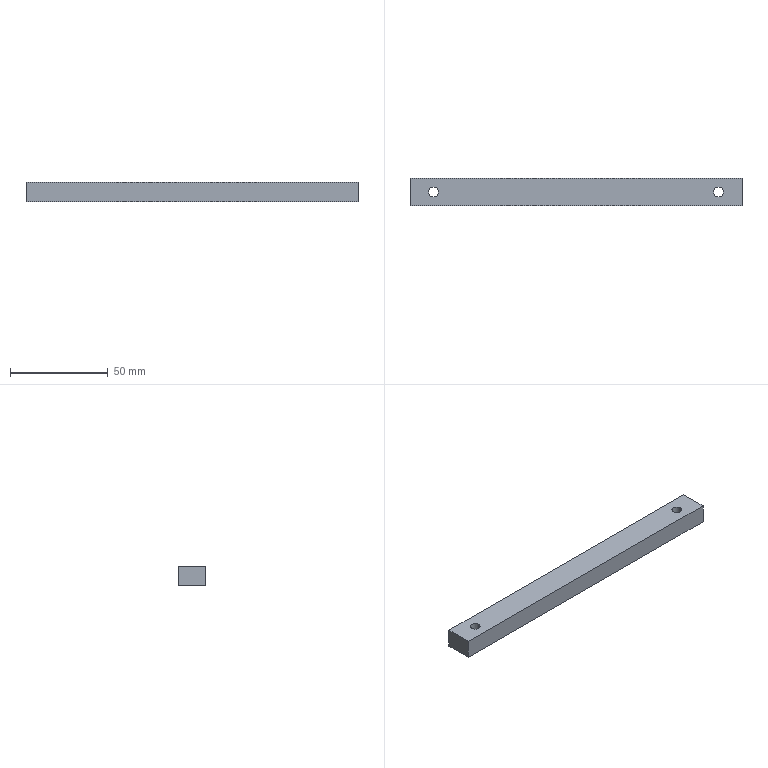Part | SolidWorks | features 3DProfileFeature 1, Extrusion 1, HoleWzd 1, MirrorPattern 1 | 1 solid | 14 faces | box 170 x 14 x 10 mm | volume 23403 mm3 | plane 6 | cone 4 | cylinder 4 | commonest cylinder face diameters 5 x4
STEP:
#1=CARTESIAN_POINT('',(75.5,0.,-4.475));
#2=VERTEX_POINT('',#1);
#3=CARTESIAN_POINT('',(70.5,0.,-4.475));
#4=VERTEX_POINT('',#3);
#5=CARTESIAN_POINT('',(73.,0.,-4.475));
#6=DIRECTION('',(0.,0.,-1.));
#7=DIRECTION('',(-1.,0.,0.));
#8=AXIS2_PLACEMENT_3D('',#5,#6,#7);
#9=CIRCLE('',#8,2.5);
#10=EDGE_CURVE('',#2,#4,#9,.T.);
#11=ORIENTED_EDGE('',*,*,#10,.F.);
#12=CARTESIAN_POINT('',(76.025,0.,-5.));
#13=VERTEX_POINT('',#12);
#14=CARTESIAN_POINT('',(76.025,0.,-5.));
#15=DIRECTION('',(0.7071,0.,-0.7071));
#16=VECTOR('',#15,1000.);
#17=LINE('',#14,#16);
#18=EDGE_CURVE('',#2,#13,#17,.T.);
#19=ORIENTED_EDGE('',*,*,#18,.T.);
#20=CARTESIAN_POINT('',(69.975,0.,-5.));
#21=VERTEX_POINT('',#20);
#22=CARTESIAN_POINT('',(73.,0.,-5.));
#23=DIRECTION('',(0.,0.,-1.));
#24=DIRECTION('',(-1.,0.,0.));
#25=AXIS2_PLACEMENT_3D('',#22,#23,#24);
#26=CIRCLE('',#25,3.025);
#27=EDGE_CURVE('',#13,#21,#26,.T.);
#28=ORIENTED_EDGE('',*,*,#27,.T.);
#29=CARTESIAN_POINT('',(69.975,0.,-5.));
#30=DIRECTION('',(-0.7071,0.,-0.7071));
#31=VECTOR('',#30,1000.);
#32=LINE('',#29,#31);
#33=EDGE_CURVE('',#4,#21,#32,.T.);
#34=ORIENTED_EDGE('',*,*,#33,.F.);
#35=EDGE_LOOP('',(#11,#19,#28,#34));
#36=FACE_OUTER_BOUND('',#35,.T.);
#37=CARTESIAN_POINT('',(73.,0.,-5.));
#38=DIRECTION('',(0.,0.,-1.));
#39=DIRECTION('',(-1.,0.,0.));
#40=AXIS2_PLACEMENT_3D('',#37,#38,#39);
#41=CONICAL_SURFACE('',#40,3.025,0.7854);
#42=ADVANCED_FACE('',(#36),#41,.F.);
#43=CARTESIAN_POINT('',(75.5,0.,5.));
#44=VERTEX_POINT('',#43);
#45=CARTESIAN_POINT('',(70.5,0.,5.));
#46=VERTEX_POINT('',#45);
#47=CARTESIAN_POINT('',(73.,0.,5.));
#48=DIRECTION('',(0.,0.,-1.));
#49=DIRECTION('',(-1.,0.,0.));
#50=AXIS2_PLACEMENT_3D('',#47,#48,#49);
#51=CIRCLE('',#50,2.5);
#52=EDGE_CURVE('',#44,#46,#51,.T.);
#53=ORIENTED_EDGE('',*,*,#52,.F.);
#54=CARTESIAN_POINT('',(75.5,0.,-5.));
#55=DIRECTION('',(0.,0.,-1.));
#56=VECTOR('',#55,1000.);
#57=LINE('',#54,#56);
#58=EDGE_CURVE('',#44,#2,#57,.T.);
#59=ORIENTED_EDGE('',*,*,#58,.T.);
#60=ORIENTED_EDGE('',*,*,#10,.T.);
#61=CARTESIAN_POINT('',(70.5,0.,-5.));
#62=DIRECTION('',(0.,0.,-1.));
#63=VECTOR('',#62,1000.);
#64=LINE('',#61,#63);
#65=EDGE_CURVE('',#46,#4,#64,.T.);
#66=ORIENTED_EDGE('',*,*,#65,.F.);
#67=EDGE_LOOP('',(#53,#59,#60,#66));
#68=FACE_OUTER_BOUND('',#67,.T.);
#69=CARTESIAN_POINT('',(73.,0.,-5.));
#70=DIRECTION('',(0.,0.,-1.));
#71=DIRECTION('',(-1.,0.,0.));
#72=AXIS2_PLACEMENT_3D('',#69,#70,#71);
#73=CYLINDRICAL_SURFACE('',#72,2.5);
#74=ADVANCED_FACE('',(#68),#73,.F.);
#75=CARTESIAN_POINT('',(-70.5,0.,-4.475));
#76=VERTEX_POINT('',#75);
#77=CARTESIAN_POINT('',(-75.5,0.,-4.475));
#78=VERTEX_POINT('',#77);
#79=CARTESIAN_POINT('',(-73.,0.,-4.475));
#80=DIRECTION('',(0.,0.,-1.));
#81=DIRECTION('',(-1.,0.,0.));
#82=AXIS2_PLACEMENT_3D('',#79,#80,#81);
#83=CIRCLE('',#82,2.5);
#84=EDGE_CURVE('',#76,#78,#83,.T.);
#85=ORIENTED_EDGE('',*,*,#84,.F.);
#86=CARTESIAN_POINT('',(-69.975,0.,-5.));
#87=VERTEX_POINT('',#86);
#88=CARTESIAN_POINT('',(-69.975,0.,-5.));
#89=DIRECTION('',(0.7071,0.,-0.7071));
#90=VECTOR('',#89,1000.);
#91=LINE('',#88,#90);
#92=EDGE_CURVE('',#76,#87,#91,.T.);
#93=ORIENTED_EDGE('',*,*,#92,.T.);
#94=CARTESIAN_POINT('',(-76.025,0.,-5.));
#95=VERTEX_POINT('',#94);
#96=CARTESIAN_POINT('',(-73.,0.,-5.));
#97=DIRECTION('',(0.,0.,-1.));
#98=DIRECTION('',(-1.,0.,0.));
#99=AXIS2_PLACEMENT_3D('',#96,#97,#98);
#100=CIRCLE('',#99,3.025);
#101=EDGE_CURVE('',#87,#95,#100,.T.);
#102=ORIENTED_EDGE('',*,*,#101,.T.);
#103=CARTESIAN_POINT('',(-76.025,0.,-5.));
#104=DIRECTION('',(-0.7071,0.,-0.7071));
#105=VECTOR('',#104,1000.);
#106=LINE('',#103,#105);
#107=EDGE_CURVE('',#78,#95,#106,.T.);
#108=ORIENTED_EDGE('',*,*,#107,.F.);
#109=EDGE_LOOP('',(#85,#93,#102,#108));
#110=FACE_OUTER_BOUND('',#109,.T.);
#111=CARTESIAN_POINT('',(-73.,0.,-5.));
#112=DIRECTION('',(0.,0.,-1.));
#113=DIRECTION('',(-1.,0.,0.));
#114=AXIS2_PLACEMENT_3D('',#111,#112,#113);
#115=CONICAL_SURFACE('',#114,3.025,0.7854);
#116=ADVANCED_FACE('',(#110),#115,.F.);
#117=CARTESIAN_POINT('',(-70.5,0.,5.));
#118=VERTEX_POINT('',#117);
#119=CARTESIAN_POINT('',(-75.5,0.,5.));
#120=VERTEX_POINT('',#119);
#121=CARTESIAN_POINT('',(-73.,0.,5.));
#122=DIRECTION('',(0.,0.,-1.));
#123=DIRECTION('',(-1.,0.,0.));
#124=AXIS2_PLACEMENT_3D('',#121,#122,#123);
#125=CIRCLE('',#124,2.5);
#126=EDGE_CURVE('',#118,#120,#125,.T.);
#127=ORIENTED_EDGE('',*,*,#126,.F.);
#128=CARTESIAN_POINT('',(-70.5,0.,-5.));
#129=DIRECTION('',(0.,0.,-1.));
#130=VECTOR('',#129,1000.);
#131=LINE('',#128,#130);
#132=EDGE_CURVE('',#118,#76,#131,.T.);
#133=ORIENTED_EDGE('',*,*,#132,.T.);
#134=ORIENTED_EDGE('',*,*,#84,.T.);
#135=CARTESIAN_POINT('',(-75.5,0.,-5.));
#136=DIRECTION('',(0.,0.,-1.));
#137=VECTOR('',#136,1000.);
#138=LINE('',#135,#137);
#139=EDGE_CURVE('',#120,#78,#138,.T.);
#140=ORIENTED_EDGE('',*,*,#139,.F.);
#141=EDGE_LOOP('',(#127,#133,#134,#140));
#142=FACE_OUTER_BOUND('',#141,.T.);
#143=CARTESIAN_POINT('',(-73.,0.,-5.));
#144=DIRECTION('',(0.,0.,-1.));
#145=DIRECTION('',(-1.,0.,0.));
#146=AXIS2_PLACEMENT_3D('',#143,#144,#145);
#147=CYLINDRICAL_SURFACE('',#146,2.5);
#148=ADVANCED_FACE('',(#142),#147,.F.);
#149=CARTESIAN_POINT('',(85.,-7.,-5.));
#150=VERTEX_POINT('',#149);
#151=CARTESIAN_POINT('',(85.,7.,-5.));
#152=VERTEX_POINT('',#151);
#153=CARTESIAN_POINT('',(85.,-7.,-5.));
#154=DIRECTION('',(0.,1.,0.));
#155=VECTOR('',#154,1000.);
#156=LINE('',#153,#155);
#157=EDGE_CURVE('',#150,#152,#156,.T.);
#158=ORIENTED_EDGE('',*,*,#157,.T.);
#159=CARTESIAN_POINT('',(85.,7.,5.));
#160=VERTEX_POINT('',#159);
#161=CARTESIAN_POINT('',(85.,7.,5.));
#162=DIRECTION('',(0.,0.,-1.));
#163=VECTOR('',#162,1000.);
#164=LINE('',#161,#163);
#165=EDGE_CURVE('',#160,#152,#164,.T.);
#166=ORIENTED_EDGE('',*,*,#165,.F.);
#167=CARTESIAN_POINT('',(85.,-7.,5.));
#168=VERTEX_POINT('',#167);
#169=CARTESIAN_POINT('',(85.,-7.,5.));
#170=DIRECTION('',(0.,1.,0.));
#171=VECTOR('',#170,1000.);
#172=LINE('',#169,#171);
#173=EDGE_CURVE('',#168,#160,#172,.T.);
#174=ORIENTED_EDGE('',*,*,#173,.F.);
#175=CARTESIAN_POINT('',(85.,-7.,5.));
#176=DIRECTION('',(0.,0.,-1.));
#177=VECTOR('',#176,1000.);
#178=LINE('',#175,#177);
#179=EDGE_CURVE('',#168,#150,#178,.T.);
#180=ORIENTED_EDGE('',*,*,#179,.T.);
#181=EDGE_LOOP('',(#158,#166,#174,#180));
#182=FACE_OUTER_BOUND('',#181,.T.);
#183=CARTESIAN_POINT('',(85.,-7.,5.));
#184=DIRECTION('',(-1.,0.,0.));
#185=DIRECTION('',(0.,0.,1.));
#186=AXIS2_PLACEMENT_3D('',#183,#184,#185);
#187=PLANE('',#186);
#188=ADVANCED_FACE('',(#182),#187,.F.);
#189=CARTESIAN_POINT('',(-85.,7.,-5.));
#190=VERTEX_POINT('',#189);
#191=CARTESIAN_POINT('',(-85.,7.,-5.));
#192=DIRECTION('',(-1.,0.,0.));
#193=VECTOR('',#192,1000.);
#194=LINE('',#191,#193);
#195=EDGE_CURVE('',#152,#190,#194,.T.);
#196=ORIENTED_EDGE('',*,*,#195,.T.);
#197=CARTESIAN_POINT('',(-85.,7.,5.));
#198=VERTEX_POINT('',#197);
#199=CARTESIAN_POINT('',(-85.,7.,5.));
#200=DIRECTION('',(0.,0.,-1.));
#201=VECTOR('',#200,1000.);
#202=LINE('',#199,#201);
#203=EDGE_CURVE('',#198,#190,#202,.T.);
#204=ORIENTED_EDGE('',*,*,#203,.F.);
#205=CARTESIAN_POINT('',(-85.,7.,5.));
#206=DIRECTION('',(-1.,0.,0.));
#207=VECTOR('',#206,1000.);
#208=LINE('',#205,#207);
#209=EDGE_CURVE('',#160,#198,#208,.T.);
#210=ORIENTED_EDGE('',*,*,#209,.F.);
#211=ORIENTED_EDGE('',*,*,#165,.T.);
#212=EDGE_LOOP('',(#196,#204,#210,#211));
#213=FACE_OUTER_BOUND('',#212,.T.);
#214=CARTESIAN_POINT('',(-85.,7.,5.));
#215=DIRECTION('',(0.,-1.,0.));
#216=DIRECTION('',(0.,0.,-1.));
#217=AXIS2_PLACEMENT_3D('',#214,#215,#216);
#218=PLANE('',#217);
#219=ADVANCED_FACE('',(#213),#218,.F.);
#220=CARTESIAN_POINT('',(-85.,-7.,-5.));
#221=VERTEX_POINT('',#220);
#222=CARTESIAN_POINT('',(-85.,-7.,-5.));
#223=DIRECTION('',(0.,-1.,0.));
#224=VECTOR('',#223,1000.);
#225=LINE('',#222,#224);
#226=EDGE_CURVE('',#190,#221,#225,.T.);
#227=ORIENTED_EDGE('',*,*,#226,.T.);
#228=CARTESIAN_POINT('',(-85.,-7.,5.));
#229=VERTEX_POINT('',#228);
#230=CARTESIAN_POINT('',(-85.,-7.,5.));
#231=DIRECTION('',(0.,0.,-1.));
#232=VECTOR('',#231,1000.);
#233=LINE('',#230,#232);
#234=EDGE_CURVE('',#229,#221,#233,.T.);
#235=ORIENTED_EDGE('',*,*,#234,.F.);
#236=CARTESIAN_POINT('',(-85.,-7.,5.));
#237=DIRECTION('',(0.,-1.,0.));
#238=VECTOR('',#237,1000.);
#239=LINE('',#236,#238);
#240=EDGE_CURVE('',#198,#229,#239,.T.);
#241=ORIENTED_EDGE('',*,*,#240,.F.);
#242=ORIENTED_EDGE('',*,*,#203,.T.);
#243=EDGE_LOOP('',(#227,#235,#241,#242));
#244=FACE_OUTER_BOUND('',#243,.T.);
#245=CARTESIAN_POINT('',(-85.,-7.,5.));
#246=DIRECTION('',(1.,0.,0.));
#247=DIRECTION('',(0.,0.,-1.));
#248=AXIS2_PLACEMENT_3D('',#245,#246,#247);
#249=PLANE('',#248);
#250=ADVANCED_FACE('',(#244),#249,.F.);
#251=CARTESIAN_POINT('',(-85.,-7.,-5.));
#252=DIRECTION('',(1.,0.,0.));
#253=VECTOR('',#252,1000.);
#254=LINE('',#251,#253);
#255=EDGE_CURVE('',#221,#150,#254,.T.);
#256=ORIENTED_EDGE('',*,*,#255,.T.);
#257=ORIENTED_EDGE('',*,*,#179,.F.);
#258=CARTESIAN_POINT('',(-85.,-7.,5.));
#259=DIRECTION('',(1.,0.,0.));
#260=VECTOR('',#259,1000.);
#261=LINE('',#258,#260);
#262=EDGE_CURVE('',#229,#168,#261,.T.);
#263=ORIENTED_EDGE('',*,*,#262,.F.);
#264=ORIENTED_EDGE('',*,*,#234,.T.);
#265=EDGE_LOOP('',(#256,#257,#263,#264));
#266=FACE_OUTER_BOUND('',#265,.T.);
#267=CARTESIAN_POINT('',(-85.,-7.,5.));
#268=DIRECTION('',(0.,1.,0.));
#269=DIRECTION('',(0.,0.,1.));
#270=AXIS2_PLACEMENT_3D('',#267,#268,#269);
#271=PLANE('',#270);
#272=ADVANCED_FACE('',(#266),#271,.F.);
#273=CARTESIAN_POINT('',(73.,0.,5.));
#274=DIRECTION('',(0.,0.,-1.));
#275=DIRECTION('',(-1.,0.,0.));
#276=AXIS2_PLACEMENT_3D('',#273,#274,#275);
#277=CIRCLE('',#276,2.5);
#278=EDGE_CURVE('',#46,#44,#277,.T.);
#279=ORIENTED_EDGE('',*,*,#278,.T.);
#280=ORIENTED_EDGE('',*,*,#52,.T.);
#281=EDGE_LOOP('',(#279,#280));
#282=FACE_BOUND('',#281,.T.);
#283=CARTESIAN_POINT('',(-73.,0.,5.));
#284=DIRECTION('',(0.,0.,-1.));
#285=DIRECTION('',(-1.,0.,0.));
#286=AXIS2_PLACEMENT_3D('',#283,#284,#285);
#287=CIRCLE('',#286,2.5);
#288=EDGE_CURVE('',#120,#118,#287,.T.);
#289=ORIENTED_EDGE('',*,*,#288,.T.);
#290=ORIENTED_EDGE('',*,*,#126,.T.);
#291=EDGE_LOOP('',(#289,#290));
#292=FACE_BOUND('',#291,.T.);
#293=ORIENTED_EDGE('',*,*,#173,.T.);
#294=ORIENTED_EDGE('',*,*,#209,.T.);
#295=ORIENTED_EDGE('',*,*,#240,.T.);
#296=ORIENTED_EDGE('',*,*,#262,.T.);
#297=EDGE_LOOP('',(#293,#294,#295,#296));
#298=FACE_OUTER_BOUND('',#297,.T.);
#299=CARTESIAN_POINT('',(0.,0.,5.));
#300=DIRECTION('',(0.,0.,-1.));
#301=DIRECTION('',(-1.,0.,0.));
#302=AXIS2_PLACEMENT_3D('',#299,#300,#301);
#303=PLANE('',#302);
#304=ADVANCED_FACE('',(#282,#292,#298),#303,.F.);
#305=CARTESIAN_POINT('',(73.,0.,-5.));
#306=DIRECTION('',(0.,0.,-1.));
#307=DIRECTION('',(-1.,0.,0.));
#308=AXIS2_PLACEMENT_3D('',#305,#306,#307);
#309=CIRCLE('',#308,3.025);
#310=EDGE_CURVE('',#21,#13,#309,.T.);
#311=ORIENTED_EDGE('',*,*,#310,.F.);
#312=ORIENTED_EDGE('',*,*,#27,.F.);
#313=EDGE_LOOP('',(#311,#312));
#314=FACE_BOUND('',#313,.T.);
#315=CARTESIAN_POINT('',(-73.,0.,-5.));
#316=DIRECTION('',(0.,0.,-1.));
#317=DIRECTION('',(-1.,0.,0.));
#318=AXIS2_PLACEMENT_3D('',#315,#316,#317);
#319=CIRCLE('',#318,3.025);
#320=EDGE_CURVE('',#95,#87,#319,.T.);
#321=ORIENTED_EDGE('',*,*,#320,.F.);
#322=ORIENTED_EDGE('',*,*,#101,.F.);
#323=EDGE_LOOP('',(#321,#322));
#324=FACE_BOUND('',#323,.T.);
#325=ORIENTED_EDGE('',*,*,#157,.F.);
#326=ORIENTED_EDGE('',*,*,#255,.F.);
#327=ORIENTED_EDGE('',*,*,#226,.F.);
#328=ORIENTED_EDGE('',*,*,#195,.F.);
#329=EDGE_LOOP('',(#325,#326,#327,#328));
#330=FACE_OUTER_BOUND('',#329,.T.);
#331=CARTESIAN_POINT('',(0.,0.,-5.));
#332=DIRECTION('',(0.,0.,-1.));
#333=DIRECTION('',(-1.,0.,0.));
#334=AXIS2_PLACEMENT_3D('',#331,#332,#333);
#335=PLANE('',#334);
#336=ADVANCED_FACE('',(#314,#324,#330),#335,.T.);
#337=ORIENTED_EDGE('',*,*,#132,.F.);
#338=ORIENTED_EDGE('',*,*,#288,.F.);
#339=ORIENTED_EDGE('',*,*,#139,.T.);
#340=CARTESIAN_POINT('',(-73.,0.,-4.475));
#341=DIRECTION('',(0.,0.,-1.));
#342=DIRECTION('',(-1.,0.,0.));
#343=AXIS2_PLACEMENT_3D('',#340,#341,#342);
#344=CIRCLE('',#343,2.5);
#345=EDGE_CURVE('',#78,#76,#344,.T.);
#346=ORIENTED_EDGE('',*,*,#345,.T.);
#347=EDGE_LOOP('',(#337,#338,#339,#346));
#348=FACE_OUTER_BOUND('',#347,.T.);
#349=CARTESIAN_POINT('',(-73.,0.,-5.));
#350=DIRECTION('',(0.,0.,-1.));
#351=DIRECTION('',(-1.,0.,0.));
#352=AXIS2_PLACEMENT_3D('',#349,#350,#351);
#353=CYLINDRICAL_SURFACE('',#352,2.5);
#354=ADVANCED_FACE('',(#348),#353,.F.);
#355=ORIENTED_EDGE('',*,*,#92,.F.);
#356=ORIENTED_EDGE('',*,*,#345,.F.);
#357=ORIENTED_EDGE('',*,*,#107,.T.);
#358=ORIENTED_EDGE('',*,*,#320,.T.);
#359=EDGE_LOOP('',(#355,#356,#357,#358));
#360=FACE_OUTER_BOUND('',#359,.T.);
#361=CARTESIAN_POINT('',(-73.,0.,-5.));
#362=DIRECTION('',(0.,0.,-1.));
#363=DIRECTION('',(-1.,0.,0.));
#364=AXIS2_PLACEMENT_3D('',#361,#362,#363);
#365=CONICAL_SURFACE('',#364,3.025,0.7854);
#366=ADVANCED_FACE('',(#360),#365,.F.);
#367=ORIENTED_EDGE('',*,*,#58,.F.);
#368=ORIENTED_EDGE('',*,*,#278,.F.);
#369=ORIENTED_EDGE('',*,*,#65,.T.);
#370=CARTESIAN_POINT('',(73.,0.,-4.475));
#371=DIRECTION('',(0.,0.,-1.));
#372=DIRECTION('',(-1.,0.,0.));
#373=AXIS2_PLACEMENT_3D('',#370,#371,#372);
#374=CIRCLE('',#373,2.5);
#375=EDGE_CURVE('',#4,#2,#374,.T.);
#376=ORIENTED_EDGE('',*,*,#375,.T.);
#377=EDGE_LOOP('',(#367,#368,#369,#376));
#378=FACE_OUTER_BOUND('',#377,.T.);
#379=CARTESIAN_POINT('',(73.,0.,-5.));
#380=DIRECTION('',(0.,0.,-1.));
#381=DIRECTION('',(-1.,0.,0.));
#382=AXIS2_PLACEMENT_3D('',#379,#380,#381);
#383=CYLINDRICAL_SURFACE('',#382,2.5);
#384=ADVANCED_FACE('',(#378),#383,.F.);
#385=ORIENTED_EDGE('',*,*,#18,.F.);
#386=ORIENTED_EDGE('',*,*,#375,.F.);
#387=ORIENTED_EDGE('',*,*,#33,.T.);
#388=ORIENTED_EDGE('',*,*,#310,.T.);
#389=EDGE_LOOP('',(#385,#386,#387,#388));
#390=FACE_OUTER_BOUND('',#389,.T.);
#391=CARTESIAN_POINT('',(73.,0.,-5.));
#392=DIRECTION('',(0.,0.,-1.));
#393=DIRECTION('',(-1.,0.,0.));
#394=AXIS2_PLACEMENT_3D('',#391,#392,#393);
#395=CONICAL_SURFACE('',#394,3.025,0.7854);
#396=ADVANCED_FACE('',(#390),#395,.F.);
#397=CLOSED_SHELL('',(#42,#74,#116,#148,#188,#219,#250,#272,#304,#336,#354,#366,#384,#396));
#398=MANIFOLD_SOLID_BREP('',#397);
#399=CARTESIAN_POINT('',(0.,0.,0.));
#400=DIRECTION('',(0.,0.,1.));
#401=DIRECTION('',(1.,0.,0.));
#402=AXIS2_PLACEMENT_3D('',#399,#400,#401);
#403=(LENGTH_UNIT()NAMED_UNIT(*)SI_UNIT(.MILLI.,.METRE.));
#404=UNCERTAINTY_MEASURE_WITH_UNIT(LENGTH_MEASURE(0.00001),#403,'','');
#405=(NAMED_UNIT(*)PLANE_ANGLE_UNIT()SI_UNIT($,.RADIAN.));
#406=(NAMED_UNIT(*)SI_UNIT($,.STERADIAN.)SOLID_ANGLE_UNIT());
#407=(GEOMETRIC_REPRESENTATION_CONTEXT(3)GLOBAL_UNCERTAINTY_ASSIGNED_CONTEXT((#404))GLOBAL_UNIT_ASSIGNED_CONTEXT((#403,#405,#406))REPRESENTATION_CONTEXT('',''));
#408=ADVANCED_BREP_SHAPE_REPRESENTATION('',(#398,#402),#407);